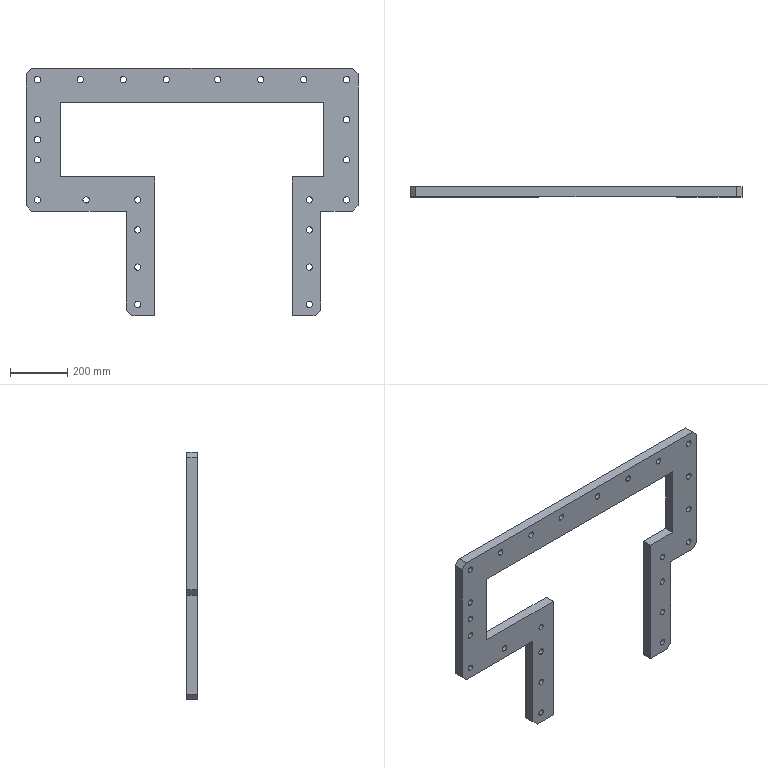Part | SolidWorks | features ICE 2, Chamfer 1, Extrusion 1 | 1 solid | 72 faces | box 1160 x 35 x 865 mm | volume 12105689 mm3 | cylinder 48 | plane 24 | commonest cylinder face diameters 22 x48